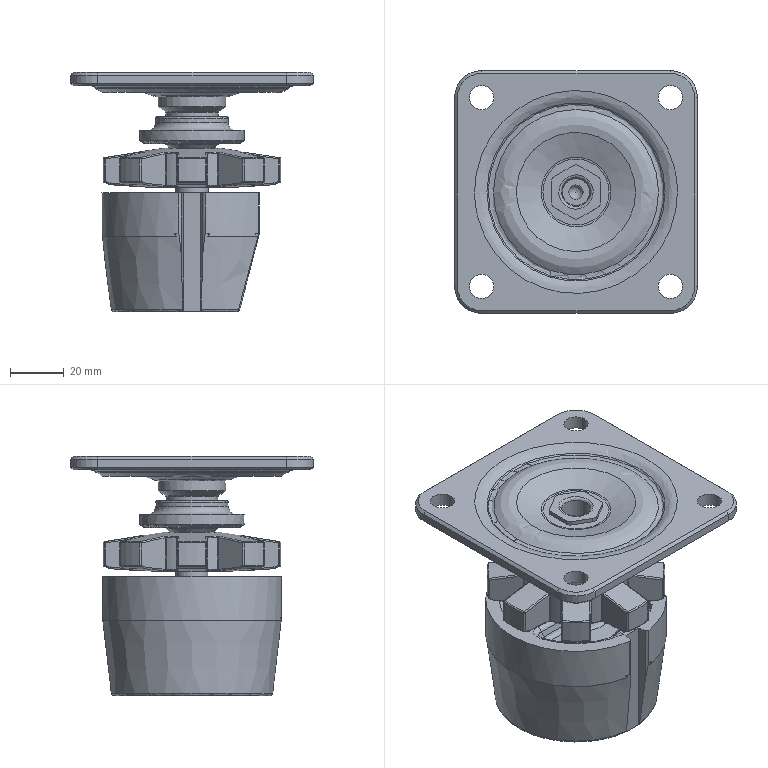Part | STEP file | 1 solid | 643 faces | box 90 x 90 x 88.64 mm | volume 185053 mm3 | spline 237 | plane 183 | cylinder 146 | cone 66 | torus 10 | other 1 | commonest cylinder face diameters 4 x52 1 x32 2 x11 40 x8 66 x8 57 x6